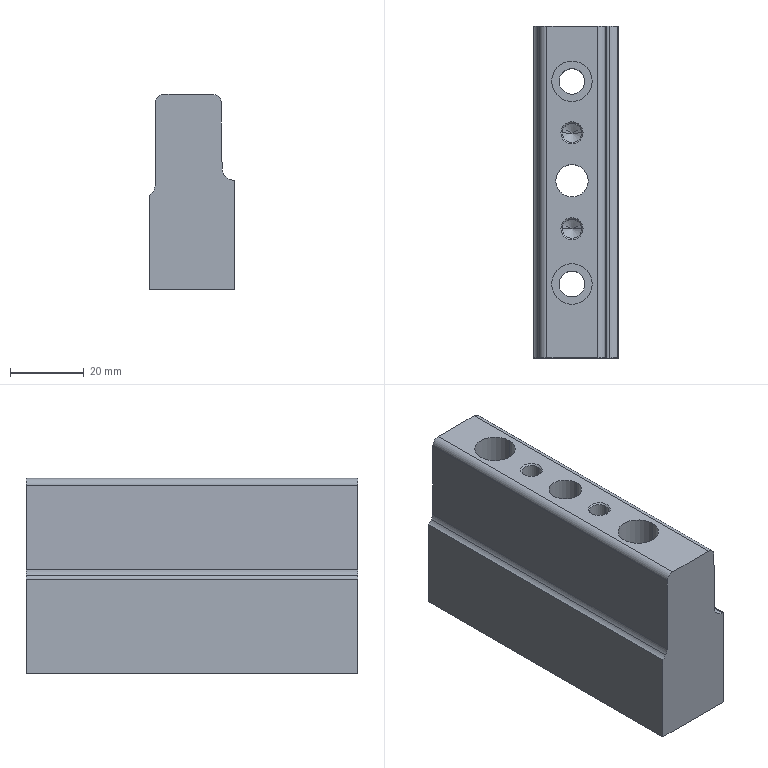Part | 1 solid | 43 faces | box 23.278 x 90 x 52.95 mm | volume 88690 mm3 | cylinder 23 | plane 12 | cone 8 | commonest cylinder face diameters 11 x6 5.2 x4 7 x4 4 x2 6.648 x2 8.8 x2